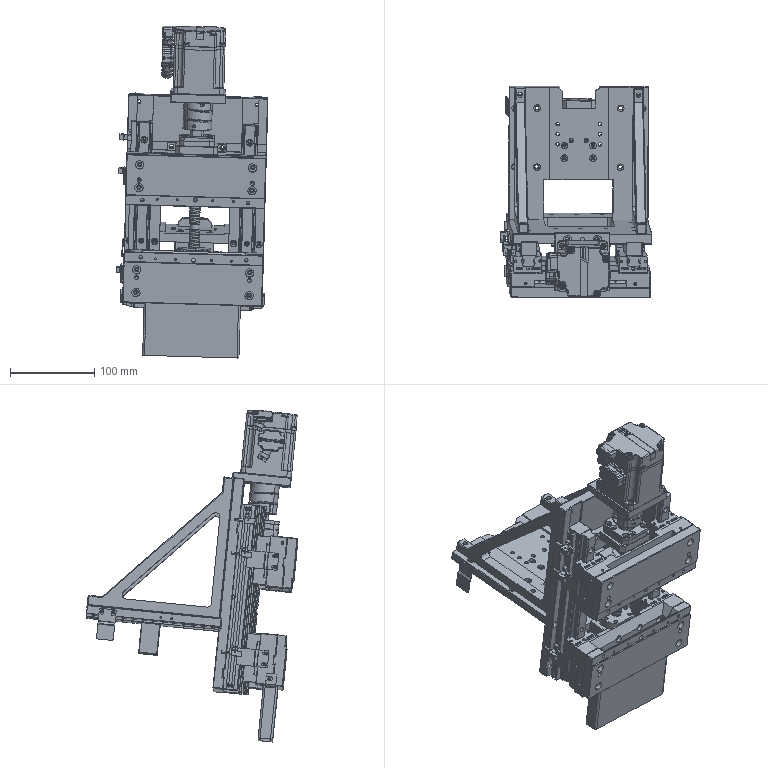Part | SolidWorks | 44 solids | 7367 faces | volume 1570886 mm3 | plane 4077 | cylinder 2095 | spline 672 | cone 480 | torus 43 | commonest cylinder face diameters 3.3 x152 4.5 x130 0.6 x106 2.5 x106 1 x105 8 x105